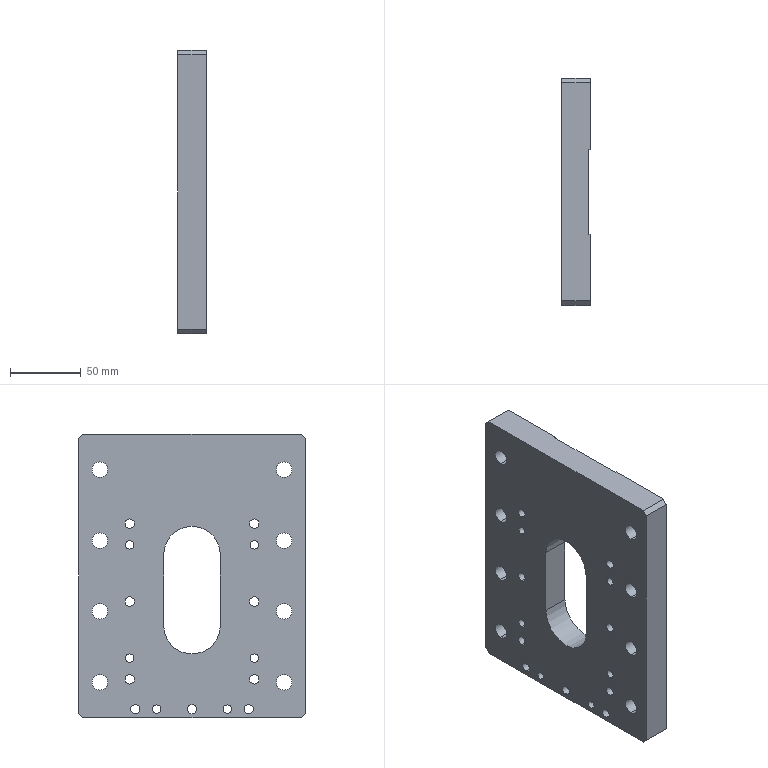Part | SolidWorks | features HoleWzd 2, ICE 2, Chamfer 1 | 1 solid | 92 faces | box 20 x 160 x 200 mm | volume 537437 mm3 | cylinder 67 | plane 25 | commonest cylinder face diameters 11 x34 6.6 x18 6 x12 40 x3